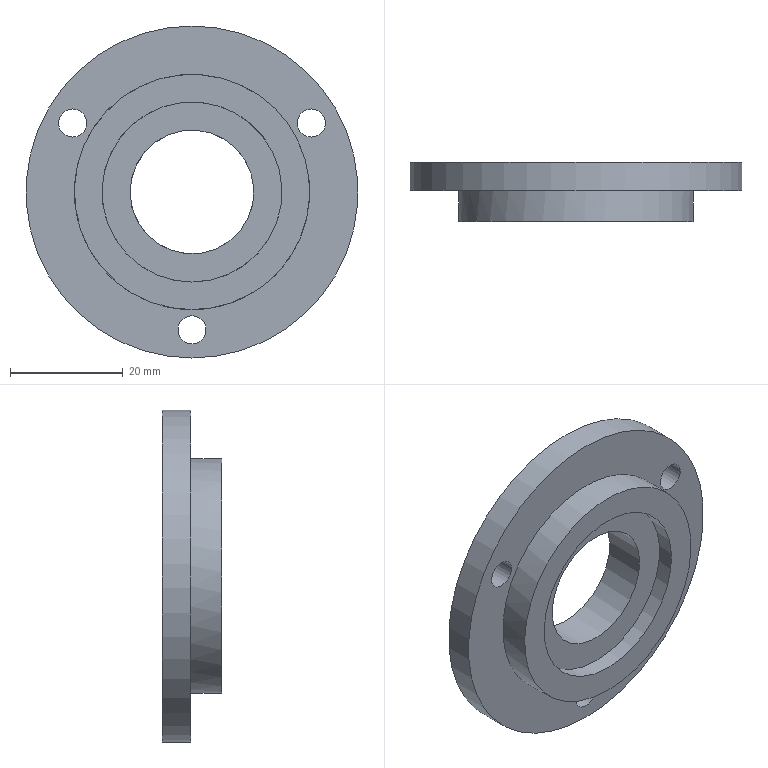Part | STEP file | YBQDJ-YB-13 | 1 solid | 11 faces | box 59 x 10.5 x 59 mm | volume 15659 mm3 | cylinder 7 | plane 4 | commonest cylinder face diameters 5 x3 22 x1 32 x1 41.8 x1 59 x1
STEP:
#1=CARTESIAN_POINT('',(0.,0.,0.));
#2=DIRECTION('',(0.,0.,1.));
#3=DIRECTION('',(1.,0.,0.));
#4=AXIS2_PLACEMENT_3D('',#1,#2,#3);
#5=CARTESIAN_POINT('',(-168.721,-90.,118.779));
#6=VERTEX_POINT('',#5);
#7=CARTESIAN_POINT('',(-183.5,-90.,104.));
#8=DIRECTION('',(0.,-1.,0.));
#9=DIRECTION('',(0.7071,0.,0.7071));
#10=AXIS2_PLACEMENT_3D('',#7,#8,#9);
#11=CIRCLE('',#10,20.9);
#12=CARTESIAN_POINT('',(-183.5,-95.,104.));
#13=DIRECTION('',(0.,1.,0.));
#14=DIRECTION('',(0.7071,0.,0.7071));
#15=AXIS2_PLACEMENT_3D('',#12,#13,#14);
#16=CYLINDRICAL_SURFACE('',#15,20.9);
#17=CARTESIAN_POINT('',(6.283,5.));
#18=DIRECTION('',(-1.,0.));
#19=VECTOR('',#18,1.);
#20=LINE('',#17,#19);
#21=(GEOMETRIC_REPRESENTATION_CONTEXT(2)PARAMETRIC_REPRESENTATION_CONTEXT()REPRESENTATION_CONTEXT('',''));
#22=DEFINITIONAL_REPRESENTATION('',(#20),#21);
#23=PCURVE('',#16,#22);
#24=CARTESIAN_POINT('',(-183.5,-90.,104.));
#25=DIRECTION('',(0.,-1.,0.));
#26=DIRECTION('',(-0.7071,0.,-0.7071));
#27=AXIS2_PLACEMENT_3D('',#24,#25,#26);
#28=PLANE('',#27);
#29=CARTESIAN_POINT('',(0.,0.));
#30=DIRECTION('',(-1.,0.));
#31=AXIS2_PLACEMENT_2D('',#29,#30);
#32=CIRCLE('',#31,20.9);
#33=(GEOMETRIC_REPRESENTATION_CONTEXT(2)PARAMETRIC_REPRESENTATION_CONTEXT()REPRESENTATION_CONTEXT('',''));
#34=DEFINITIONAL_REPRESENTATION('',(#32),#33);
#35=PCURVE('',#28,#34);
#36=SURFACE_CURVE('',#11,(#23,#35),.PCURVE_S1.);
#37=EDGE_CURVE('',#6,#6,#36,.T.);
#38=ORIENTED_EDGE('',*,*,#37,.T.);
#39=CARTESIAN_POINT('',(-168.721,-95.5,118.779));
#40=VERTEX_POINT('',#39);
#41=CARTESIAN_POINT('',(-168.721,-95.5,118.779));
#42=CARTESIAN_POINT('',(-168.721,-90.,118.779));
#43=B_SPLINE_CURVE_WITH_KNOTS('',1,(#41,#42),.UNSPECIFIED.,.F.,.F.,(2,2),(-0.5,5.),.PIECEWISE_BEZIER_KNOTS.);
#44=CARTESIAN_POINT('',(0.,0.));
#45=DIRECTION('',(0.,1.));
#46=VECTOR('',#45,1.);
#47=LINE('',#44,#46);
#48=(GEOMETRIC_REPRESENTATION_CONTEXT(2)PARAMETRIC_REPRESENTATION_CONTEXT()REPRESENTATION_CONTEXT('',''));
#49=DEFINITIONAL_REPRESENTATION('',(#47),#48);
#50=PCURVE('',#16,#49);
#51=CARTESIAN_POINT('',(6.283,0.));
#52=DIRECTION('',(0.,1.));
#53=VECTOR('',#52,1.);
#54=LINE('',#51,#53);
#55=(GEOMETRIC_REPRESENTATION_CONTEXT(2)PARAMETRIC_REPRESENTATION_CONTEXT()REPRESENTATION_CONTEXT('',''));
#56=DEFINITIONAL_REPRESENTATION('',(#54),#55);
#57=PCURVE('',#16,#56);
#58=SEAM_CURVE('',#43,(#50,#57),.PCURVE_S1.);
#59=EDGE_CURVE('',#40,#6,#58,.T.);
#60=ORIENTED_EDGE('',*,*,#59,.F.);
#61=CARTESIAN_POINT('',(-183.5,-95.5,83.1));
#62=VERTEX_POINT('',#61);
#63=CARTESIAN_POINT('',(-183.5,-95.5,104.));
#64=DIRECTION('',(0.,1.,0.));
#65=DIRECTION('',(0.,0.,-1.));
#66=AXIS2_PLACEMENT_3D('',#63,#64,#65);
#67=CIRCLE('',#66,20.9);
#68=CARTESIAN_POINT('',(-3.927,-0.5));
#69=DIRECTION('',(1.,0.));
#70=VECTOR('',#69,1.);
#71=LINE('',#68,#70);
#72=(GEOMETRIC_REPRESENTATION_CONTEXT(2)PARAMETRIC_REPRESENTATION_CONTEXT()REPRESENTATION_CONTEXT('',''));
#73=DEFINITIONAL_REPRESENTATION('',(#71),#72);
#74=PCURVE('',#16,#73);
#75=CARTESIAN_POINT('',(-183.5,-95.5,94.));
#76=DIRECTION('',(0.,1.,0.));
#77=DIRECTION('',(0.,0.,1.));
#78=AXIS2_PLACEMENT_3D('',#75,#76,#77);
#79=PLANE('',#78);
#80=CARTESIAN_POINT('',(10.,0.));
#81=DIRECTION('',(-1.,0.));
#82=AXIS2_PLACEMENT_2D('',#80,#81);
#83=CIRCLE('',#82,20.9);
#84=(GEOMETRIC_REPRESENTATION_CONTEXT(2)PARAMETRIC_REPRESENTATION_CONTEXT()REPRESENTATION_CONTEXT('',''));
#85=DEFINITIONAL_REPRESENTATION('',(#83),#84);
#86=PCURVE('',#79,#85);
#87=SURFACE_CURVE('',#67,(#74,#86),.PCURVE_S1.);
#88=EDGE_CURVE('',#40,#62,#87,.T.);
#89=ORIENTED_EDGE('',*,*,#88,.T.);
#90=CARTESIAN_POINT('',(-183.5,-95.5,104.));
#91=DIRECTION('',(0.,1.,0.));
#92=DIRECTION('',(0.,0.,-1.));
#93=AXIS2_PLACEMENT_3D('',#90,#91,#92);
#94=CIRCLE('',#93,20.9);
#95=CARTESIAN_POINT('',(2.356,-0.5));
#96=DIRECTION('',(1.,0.));
#97=VECTOR('',#96,1.);
#98=LINE('',#95,#97);
#99=(GEOMETRIC_REPRESENTATION_CONTEXT(2)PARAMETRIC_REPRESENTATION_CONTEXT()REPRESENTATION_CONTEXT('',''));
#100=DEFINITIONAL_REPRESENTATION('',(#98),#99);
#101=PCURVE('',#16,#100);
#102=CARTESIAN_POINT('',(10.,0.));
#103=DIRECTION('',(-1.,0.));
#104=AXIS2_PLACEMENT_2D('',#102,#103);
#105=CIRCLE('',#104,20.9);
#106=(GEOMETRIC_REPRESENTATION_CONTEXT(2)PARAMETRIC_REPRESENTATION_CONTEXT()REPRESENTATION_CONTEXT('',''));
#107=DEFINITIONAL_REPRESENTATION('',(#105),#106);
#108=PCURVE('',#79,#107);
#109=SURFACE_CURVE('',#94,(#101,#108),.PCURVE_S1.);
#110=EDGE_CURVE('',#62,#40,#109,.T.);
#111=ORIENTED_EDGE('',*,*,#110,.T.);
#112=ORIENTED_EDGE('',*,*,#59,.T.);
#113=EDGE_LOOP('',(#38,#60,#89,#111,#112));
#114=FACE_BOUND('',#113,.T.);
#115=ADVANCED_FACE('',(#114),#16,.T.);
#116=CARTESIAN_POINT('',(-183.5,-85.,133.5));
#117=VERTEX_POINT('',#116);
#118=CARTESIAN_POINT('',(-183.5,-85.,104.));
#119=DIRECTION('',(0.,1.,0.));
#120=DIRECTION('',(0.,0.,1.));
#121=AXIS2_PLACEMENT_3D('',#118,#119,#120);
#122=CIRCLE('',#121,29.5);
#123=CARTESIAN_POINT('',(-183.5,-85.,104.));
#124=DIRECTION('',(0.,-1.,0.));
#125=DIRECTION('',(-0.7071,0.,-0.7071));
#126=AXIS2_PLACEMENT_3D('',#123,#124,#125);
#127=CYLINDRICAL_SURFACE('',#126,29.5);
#128=CARTESIAN_POINT('',(10.21,0.));
#129=DIRECTION('',(-1.,0.));
#130=VECTOR('',#129,1.);
#131=LINE('',#128,#130);
#132=(GEOMETRIC_REPRESENTATION_CONTEXT(2)PARAMETRIC_REPRESENTATION_CONTEXT()REPRESENTATION_CONTEXT('',''));
#133=DEFINITIONAL_REPRESENTATION('',(#131),#132);
#134=PCURVE('',#127,#133);
#135=CARTESIAN_POINT('',(-183.5,-85.,104.));
#136=DIRECTION('',(0.,-1.,0.));
#137=DIRECTION('',(-0.7071,0.,-0.7071));
#138=AXIS2_PLACEMENT_3D('',#135,#136,#137);
#139=PLANE('',#138);
#140=CARTESIAN_POINT('',(-20.86,-20.86));
#141=CARTESIAN_POINT('',(-56.99,15.27));
#142=CARTESIAN_POINT('',(-7.635,28.495));
#143=CARTESIAN_POINT('',(41.719,41.719));
#144=CARTESIAN_POINT('',(28.495,-7.635));
#145=CARTESIAN_POINT('',(15.27,-56.99));
#146=CARTESIAN_POINT('',(-20.86,-20.86));
#147=(BOUNDED_CURVE()B_SPLINE_CURVE(2,(#140,#141,#142,#143,#144,#145,#146),.UNSPECIFIED.,.T.,.F.)B_SPLINE_CURVE_WITH_KNOTS((1,2,2,2,2,1),(-2.094,0.,2.094,4.189,6.283,8.378),.UNSPECIFIED.)CURVE()GEOMETRIC_REPRESENTATION_ITEM()RATIONAL_B_SPLINE_CURVE((1.,0.5,1.,0.5,1.,0.5,1.))REPRESENTATION_ITEM(''));
#148=(GEOMETRIC_REPRESENTATION_CONTEXT(2)PARAMETRIC_REPRESENTATION_CONTEXT()REPRESENTATION_CONTEXT('',''));
#149=DEFINITIONAL_REPRESENTATION('',(#147),#148);
#150=PCURVE('',#139,#149);
#151=SURFACE_CURVE('',#122,(#134,#150),.PCURVE_S1.);
#152=EDGE_CURVE('',#117,#117,#151,.T.);
#153=ORIENTED_EDGE('',*,*,#152,.F.);
#154=CARTESIAN_POINT('',(-183.5,-90.,133.5));
#155=VERTEX_POINT('',#154);
#156=CARTESIAN_POINT('',(-183.5,-85.,133.5));
#157=CARTESIAN_POINT('',(-183.5,-90.,133.5));
#158=B_SPLINE_CURVE_WITH_KNOTS('',1,(#156,#157),.UNSPECIFIED.,.F.,.F.,(2,2),(0.,5.),.PIECEWISE_BEZIER_KNOTS.);
#159=CARTESIAN_POINT('',(10.21,0.));
#160=DIRECTION('',(0.,1.));
#161=VECTOR('',#160,1.);
#162=LINE('',#159,#161);
#163=(GEOMETRIC_REPRESENTATION_CONTEXT(2)PARAMETRIC_REPRESENTATION_CONTEXT()REPRESENTATION_CONTEXT('',''));
#164=DEFINITIONAL_REPRESENTATION('',(#162),#163);
#165=PCURVE('',#127,#164);
#166=CARTESIAN_POINT('',(3.927,0.));
#167=DIRECTION('',(0.,1.));
#168=VECTOR('',#167,1.);
#169=LINE('',#166,#168);
#170=(GEOMETRIC_REPRESENTATION_CONTEXT(2)PARAMETRIC_REPRESENTATION_CONTEXT()REPRESENTATION_CONTEXT('',''));
#171=DEFINITIONAL_REPRESENTATION('',(#169),#170);
#172=PCURVE('',#127,#171);
#173=SEAM_CURVE('',#158,(#165,#172),.PCURVE_S1.);
#174=EDGE_CURVE('',#117,#155,#173,.T.);
#175=ORIENTED_EDGE('',*,*,#174,.T.);
#176=CARTESIAN_POINT('',(-183.5,-90.,104.));
#177=DIRECTION('',(0.,1.,0.));
#178=DIRECTION('',(0.,0.,1.));
#179=AXIS2_PLACEMENT_3D('',#176,#177,#178);
#180=CIRCLE('',#179,29.5);
#181=CARTESIAN_POINT('',(10.21,5.));
#182=DIRECTION('',(-1.,0.));
#183=VECTOR('',#182,1.);
#184=LINE('',#181,#183);
#185=(GEOMETRIC_REPRESENTATION_CONTEXT(2)PARAMETRIC_REPRESENTATION_CONTEXT()REPRESENTATION_CONTEXT('',''));
#186=DEFINITIONAL_REPRESENTATION('',(#184),#185);
#187=PCURVE('',#127,#186);
#188=CARTESIAN_POINT('',(-20.86,-20.86));
#189=CARTESIAN_POINT('',(-56.99,15.27));
#190=CARTESIAN_POINT('',(-7.635,28.495));
#191=CARTESIAN_POINT('',(41.719,41.719));
#192=CARTESIAN_POINT('',(28.495,-7.635));
#193=CARTESIAN_POINT('',(15.27,-56.99));
#194=CARTESIAN_POINT('',(-20.86,-20.86));
#195=(BOUNDED_CURVE()B_SPLINE_CURVE(2,(#188,#189,#190,#191,#192,#193,#194),.UNSPECIFIED.,.T.,.F.)B_SPLINE_CURVE_WITH_KNOTS((1,2,2,2,2,1),(-2.094,0.,2.094,4.189,6.283,8.378),.UNSPECIFIED.)CURVE()GEOMETRIC_REPRESENTATION_ITEM()RATIONAL_B_SPLINE_CURVE((1.,0.5,1.,0.5,1.,0.5,1.))REPRESENTATION_ITEM(''));
#196=(GEOMETRIC_REPRESENTATION_CONTEXT(2)PARAMETRIC_REPRESENTATION_CONTEXT()REPRESENTATION_CONTEXT('',''));
#197=DEFINITIONAL_REPRESENTATION('',(#195),#196);
#198=PCURVE('',#28,#197);
#199=SURFACE_CURVE('',#180,(#187,#198),.PCURVE_S1.);
#200=EDGE_CURVE('',#155,#155,#199,.T.);
#201=ORIENTED_EDGE('',*,*,#200,.T.);
#202=ORIENTED_EDGE('',*,*,#174,.F.);
#203=EDGE_LOOP('',(#153,#175,#201,#202));
#204=FACE_BOUND('',#203,.T.);
#205=ADVANCED_FACE('',(#204),#127,.T.);
#206=CARTESIAN_POINT('',(-204.718,-85.,118.75));
#207=VERTEX_POINT('',#206);
#208=CARTESIAN_POINT('',(-204.718,-85.,116.25));
#209=DIRECTION('',(0.,1.,0.));
#210=DIRECTION('',(0.,0.,1.));
#211=AXIS2_PLACEMENT_3D('',#208,#209,#210);
#212=CIRCLE('',#211,2.5);
#213=CARTESIAN_POINT('',(4.573,-25.433));
#214=CARTESIAN_POINT('',(1.511,-22.371));
#215=CARTESIAN_POINT('',(5.694,-21.25));
#216=CARTESIAN_POINT('',(9.877,-20.13));
#217=CARTESIAN_POINT('',(8.756,-24.312));
#218=CARTESIAN_POINT('',(7.635,-28.495));
#219=CARTESIAN_POINT('',(4.573,-25.433));
#220=(BOUNDED_CURVE()B_SPLINE_CURVE(2,(#213,#214,#215,#216,#217,#218,#219),.UNSPECIFIED.,.T.,.F.)B_SPLINE_CURVE_WITH_KNOTS((1,2,2,2,2,1),(-2.094,0.,2.094,4.189,6.283,8.378),.UNSPECIFIED.)CURVE()GEOMETRIC_REPRESENTATION_ITEM()RATIONAL_B_SPLINE_CURVE((1.,0.5,1.,0.5,1.,0.5,1.))REPRESENTATION_ITEM(''));
#221=(GEOMETRIC_REPRESENTATION_CONTEXT(2)PARAMETRIC_REPRESENTATION_CONTEXT()REPRESENTATION_CONTEXT('',''));
#222=DEFINITIONAL_REPRESENTATION('',(#220),#221);
#223=PCURVE('',#139,#222);
#224=CARTESIAN_POINT('',(-204.718,-97.2,116.25));
#225=DIRECTION('',(0.,1.,0.));
#226=DIRECTION('',(1.,0.,0.));
#227=AXIS2_PLACEMENT_3D('',#224,#225,#226);
#228=CYLINDRICAL_SURFACE('',#227,2.5);
#229=CARTESIAN_POINT('',(4.712,12.2));
#230=DIRECTION('',(1.,0.));
#231=VECTOR('',#230,1.);
#232=LINE('',#229,#231);
#233=(GEOMETRIC_REPRESENTATION_CONTEXT(2)PARAMETRIC_REPRESENTATION_CONTEXT()REPRESENTATION_CONTEXT('',''));
#234=DEFINITIONAL_REPRESENTATION('',(#232),#233);
#235=PCURVE('',#228,#234);
#236=SURFACE_CURVE('',#212,(#223,#235),.PCURVE_S1.);
#237=EDGE_CURVE('',#207,#207,#236,.T.);
#238=ORIENTED_EDGE('',*,*,#237,.F.);
#239=EDGE_LOOP('',(#238));
#240=FACE_BOUND('',#239,.T.);
#241=CARTESIAN_POINT('',(-183.5,-85.,82.));
#242=VERTEX_POINT('',#241);
#243=CARTESIAN_POINT('',(-183.5,-85.,79.5));
#244=DIRECTION('',(0.,1.,0.));
#245=DIRECTION('',(0.,0.,1.));
#246=AXIS2_PLACEMENT_3D('',#243,#244,#245);
#247=CIRCLE('',#246,2.5);
#248=CARTESIAN_POINT('',(15.556,15.556));
#249=CARTESIAN_POINT('',(12.494,18.618));
#250=CARTESIAN_POINT('',(16.677,19.739));
#251=CARTESIAN_POINT('',(20.86,20.86));
#252=CARTESIAN_POINT('',(19.739,16.677));
#253=CARTESIAN_POINT('',(18.618,12.494));
#254=CARTESIAN_POINT('',(15.556,15.556));
#255=(BOUNDED_CURVE()B_SPLINE_CURVE(2,(#248,#249,#250,#251,#252,#253,#254),.UNSPECIFIED.,.T.,.F.)B_SPLINE_CURVE_WITH_KNOTS((1,2,2,2,2,1),(-2.094,0.,2.094,4.189,6.283,8.378),.UNSPECIFIED.)CURVE()GEOMETRIC_REPRESENTATION_ITEM()RATIONAL_B_SPLINE_CURVE((1.,0.5,1.,0.5,1.,0.5,1.))REPRESENTATION_ITEM(''));
#256=(GEOMETRIC_REPRESENTATION_CONTEXT(2)PARAMETRIC_REPRESENTATION_CONTEXT()REPRESENTATION_CONTEXT('',''));
#257=DEFINITIONAL_REPRESENTATION('',(#255),#256);
#258=PCURVE('',#139,#257);
#259=CARTESIAN_POINT('',(-183.5,-97.2,79.5));
#260=DIRECTION('',(0.,1.,0.));
#261=DIRECTION('',(1.,0.,0.));
#262=AXIS2_PLACEMENT_3D('',#259,#260,#261);
#263=CYLINDRICAL_SURFACE('',#262,2.5);
#264=CARTESIAN_POINT('',(4.712,12.2));
#265=DIRECTION('',(1.,0.));
#266=VECTOR('',#265,1.);
#267=LINE('',#264,#266);
#268=(GEOMETRIC_REPRESENTATION_CONTEXT(2)PARAMETRIC_REPRESENTATION_CONTEXT()REPRESENTATION_CONTEXT('',''));
#269=DEFINITIONAL_REPRESENTATION('',(#267),#268);
#270=PCURVE('',#263,#269);
#271=SURFACE_CURVE('',#247,(#258,#270),.PCURVE_S1.);
#272=EDGE_CURVE('',#242,#242,#271,.T.);
#273=ORIENTED_EDGE('',*,*,#272,.F.);
#274=EDGE_LOOP('',(#273));
#275=FACE_BOUND('',#274,.T.);
#276=CARTESIAN_POINT('',(-162.282,-85.,118.75));
#277=VERTEX_POINT('',#276);
#278=CARTESIAN_POINT('',(-162.282,-85.,116.25));
#279=DIRECTION('',(0.,1.,0.));
#280=DIRECTION('',(0.,0.,1.));
#281=AXIS2_PLACEMENT_3D('',#278,#279,#280);
#282=CIRCLE('',#281,2.5);
#283=CARTESIAN_POINT('',(-25.433,4.573));
#284=CARTESIAN_POINT('',(-28.495,7.635));
#285=CARTESIAN_POINT('',(-24.312,8.756));
#286=CARTESIAN_POINT('',(-20.13,9.877));
#287=CARTESIAN_POINT('',(-21.25,5.694));
#288=CARTESIAN_POINT('',(-22.371,1.511));
#289=CARTESIAN_POINT('',(-25.433,4.573));
#290=(BOUNDED_CURVE()B_SPLINE_CURVE(2,(#283,#284,#285,#286,#287,#288,#289),.UNSPECIFIED.,.T.,.F.)B_SPLINE_CURVE_WITH_KNOTS((1,2,2,2,2,1),(-2.094,0.,2.094,4.189,6.283,8.378),.UNSPECIFIED.)CURVE()GEOMETRIC_REPRESENTATION_ITEM()RATIONAL_B_SPLINE_CURVE((1.,0.5,1.,0.5,1.,0.5,1.))REPRESENTATION_ITEM(''));
#291=(GEOMETRIC_REPRESENTATION_CONTEXT(2)PARAMETRIC_REPRESENTATION_CONTEXT()REPRESENTATION_CONTEXT('',''));
#292=DEFINITIONAL_REPRESENTATION('',(#290),#291);
#293=PCURVE('',#139,#292);
#294=CARTESIAN_POINT('',(-162.282,-97.2,116.25));
#295=DIRECTION('',(0.,1.,0.));
#296=DIRECTION('',(1.,0.,0.));
#297=AXIS2_PLACEMENT_3D('',#294,#295,#296);
#298=CYLINDRICAL_SURFACE('',#297,2.5);
#299=CARTESIAN_POINT('',(4.712,12.2));
#300=DIRECTION('',(1.,0.));
#301=VECTOR('',#300,1.);
#302=LINE('',#299,#301);
#303=(GEOMETRIC_REPRESENTATION_CONTEXT(2)PARAMETRIC_REPRESENTATION_CONTEXT()REPRESENTATION_CONTEXT('',''));
#304=DEFINITIONAL_REPRESENTATION('',(#302),#303);
#305=PCURVE('',#298,#304);
#306=SURFACE_CURVE('',#282,(#293,#305),.PCURVE_S1.);
#307=EDGE_CURVE('',#277,#277,#306,.T.);
#308=ORIENTED_EDGE('',*,*,#307,.F.);
#309=EDGE_LOOP('',(#308));
#310=FACE_BOUND('',#309,.T.);
#311=ORIENTED_EDGE('',*,*,#152,.T.);
#312=EDGE_LOOP('',(#311));
#313=FACE_BOUND('',#312,.T.);
#314=CARTESIAN_POINT('',(-175.722,-85.,111.778));
#315=VERTEX_POINT('',#314);
#316=CARTESIAN_POINT('',(-183.5,-85.,104.));
#317=DIRECTION('',(0.,-1.,0.));
#318=DIRECTION('',(0.7071,0.,0.7071));
#319=AXIS2_PLACEMENT_3D('',#316,#317,#318);
#320=CIRCLE('',#319,11.);
#321=CARTESIAN_POINT('',(0.,0.));
#322=DIRECTION('',(-1.,0.));
#323=AXIS2_PLACEMENT_2D('',#321,#322);
#324=CIRCLE('',#323,11.);
#325=(GEOMETRIC_REPRESENTATION_CONTEXT(2)PARAMETRIC_REPRESENTATION_CONTEXT()REPRESENTATION_CONTEXT('',''));
#326=DEFINITIONAL_REPRESENTATION('',(#324),#325);
#327=PCURVE('',#139,#326);
#328=CARTESIAN_POINT('',(-183.5,-95.,104.));
#329=DIRECTION('',(0.,1.,0.));
#330=DIRECTION('',(0.7071,0.,0.7071));
#331=AXIS2_PLACEMENT_3D('',#328,#329,#330);
#332=CYLINDRICAL_SURFACE('',#331,11.);
#333=CARTESIAN_POINT('',(6.283,10.));
#334=DIRECTION('',(-1.,0.));
#335=VECTOR('',#334,1.);
#336=LINE('',#333,#335);
#337=(GEOMETRIC_REPRESENTATION_CONTEXT(2)PARAMETRIC_REPRESENTATION_CONTEXT()REPRESENTATION_CONTEXT('',''));
#338=DEFINITIONAL_REPRESENTATION('',(#336),#337);
#339=PCURVE('',#332,#338);
#340=SURFACE_CURVE('',#320,(#327,#339),.PCURVE_S1.);
#341=EDGE_CURVE('',#315,#315,#340,.T.);
#342=ORIENTED_EDGE('',*,*,#341,.T.);
#343=EDGE_LOOP('',(#342));
#344=FACE_BOUND('',#343,.T.);
#345=ADVANCED_FACE('',(#240,#275,#310,#313,#344),#139,.F.);
#346=CARTESIAN_POINT('',(-204.718,-90.,118.75));
#347=VERTEX_POINT('',#346);
#348=CARTESIAN_POINT('',(-204.718,-90.,116.25));
#349=DIRECTION('',(0.,1.,0.));
#350=DIRECTION('',(0.,0.,1.));
#351=AXIS2_PLACEMENT_3D('',#348,#349,#350);
#352=CIRCLE('',#351,2.5);
#353=CARTESIAN_POINT('',(4.573,-25.433));
#354=CARTESIAN_POINT('',(1.511,-22.371));
#355=CARTESIAN_POINT('',(5.694,-21.25));
#356=CARTESIAN_POINT('',(9.877,-20.13));
#357=CARTESIAN_POINT('',(8.756,-24.312));
#358=CARTESIAN_POINT('',(7.635,-28.495));
#359=CARTESIAN_POINT('',(4.573,-25.433));
#360=(BOUNDED_CURVE()B_SPLINE_CURVE(2,(#353,#354,#355,#356,#357,#358,#359),.UNSPECIFIED.,.T.,.F.)B_SPLINE_CURVE_WITH_KNOTS((1,2,2,2,2,1),(-2.094,0.,2.094,4.189,6.283,8.378),.UNSPECIFIED.)CURVE()GEOMETRIC_REPRESENTATION_ITEM()RATIONAL_B_SPLINE_CURVE((1.,0.5,1.,0.5,1.,0.5,1.))REPRESENTATION_ITEM(''));
#361=(GEOMETRIC_REPRESENTATION_CONTEXT(2)PARAMETRIC_REPRESENTATION_CONTEXT()REPRESENTATION_CONTEXT('',''));
#362=DEFINITIONAL_REPRESENTATION('',(#360),#361);
#363=PCURVE('',#28,#362);
#364=CARTESIAN_POINT('',(4.712,7.2));
#365=DIRECTION('',(1.,0.));
#366=VECTOR('',#365,1.);
#367=LINE('',#364,#366);
#368=(GEOMETRIC_REPRESENTATION_CONTEXT(2)PARAMETRIC_REPRESENTATION_CONTEXT()REPRESENTATION_CONTEXT('',''));
#369=DEFINITIONAL_REPRESENTATION('',(#367),#368);
#370=PCURVE('',#228,#369);
#371=SURFACE_CURVE('',#352,(#363,#370),.PCURVE_S1.);
#372=EDGE_CURVE('',#347,#347,#371,.T.);
#373=ORIENTED_EDGE('',*,*,#372,.T.);
#374=EDGE_LOOP('',(#373));
#375=FACE_BOUND('',#374,.T.);
#376=CARTESIAN_POINT('',(-183.5,-90.,82.));
#377=VERTEX_POINT('',#376);
#378=CARTESIAN_POINT('',(-183.5,-90.,79.5));
#379=DIRECTION('',(0.,1.,0.));
#380=DIRECTION('',(0.,0.,1.));
#381=AXIS2_PLACEMENT_3D('',#378,#379,#380);
#382=CIRCLE('',#381,2.5);
#383=CARTESIAN_POINT('',(15.556,15.556));
#384=CARTESIAN_POINT('',(12.494,18.618));
#385=CARTESIAN_POINT('',(16.677,19.739));
#386=CARTESIAN_POINT('',(20.86,20.86));
#387=CARTESIAN_POINT('',(19.739,16.677));
#388=CARTESIAN_POINT('',(18.618,12.494));
#389=CARTESIAN_POINT('',(15.556,15.556));
#390=(BOUNDED_CURVE()B_SPLINE_CURVE(2,(#383,#384,#385,#386,#387,#388,#389),.UNSPECIFIED.,.T.,.F.)B_SPLINE_CURVE_WITH_KNOTS((1,2,2,2,2,1),(-2.094,0.,2.094,4.189,6.283,8.378),.UNSPECIFIED.)CURVE()GEOMETRIC_REPRESENTATION_ITEM()RATIONAL_B_SPLINE_CURVE((1.,0.5,1.,0.5,1.,0.5,1.))REPRESENTATION_ITEM(''));
#391=(GEOMETRIC_REPRESENTATION_CONTEXT(2)PARAMETRIC_REPRESENTATION_CONTEXT()REPRESENTATION_CONTEXT('',''));
#392=DEFINITIONAL_REPRESENTATION('',(#390),#391);
#393=PCURVE('',#28,#392);
#394=CARTESIAN_POINT('',(4.712,7.2));
#395=DIRECTION('',(1.,0.));
#396=VECTOR('',#395,1.);
#397=LINE('',#394,#396);
#398=(GEOMETRIC_REPRESENTATION_CONTEXT(2)PARAMETRIC_REPRESENTATION_CONTEXT()REPRESENTATION_CONTEXT('',''));
#399=DEFINITIONAL_REPRESENTATION('',(#397),#398);
#400=PCURVE('',#263,#399);
#401=SURFACE_CURVE('',#382,(#393,#400),.PCURVE_S1.);
#402=EDGE_CURVE('',#377,#377,#401,.T.);
#403=ORIENTED_EDGE('',*,*,#402,.T.);
#404=EDGE_LOOP('',(#403));
#405=FACE_BOUND('',#404,.T.);
#406=CARTESIAN_POINT('',(-162.282,-90.,118.75));
#407=VERTEX_POINT('',#406);
#408=CARTESIAN_POINT('',(-162.282,-90.,116.25));
#409=DIRECTION('',(0.,1.,0.));
#410=DIRECTION('',(0.,0.,1.));
#411=AXIS2_PLACEMENT_3D('',#408,#409,#410);
#412=CIRCLE('',#411,2.5);
#413=CARTESIAN_POINT('',(-25.433,4.573));
#414=CARTESIAN_POINT('',(-28.495,7.635));
#415=CARTESIAN_POINT('',(-24.312,8.756));
#416=CARTESIAN_POINT('',(-20.13,9.877));
#417=CARTESIAN_POINT('',(-21.25,5.694));
#418=CARTESIAN_POINT('',(-22.371,1.511));
#419=CARTESIAN_POINT('',(-25.433,4.573));
#420=(BOUNDED_CURVE()B_SPLINE_CURVE(2,(#413,#414,#415,#416,#417,#418,#419),.UNSPECIFIED.,.T.,.F.)B_SPLINE_CURVE_WITH_KNOTS((1,2,2,2,2,1),(-2.094,0.,2.094,4.189,6.283,8.378),.UNSPECIFIED.)CURVE()GEOMETRIC_REPRESENTATION_ITEM()RATIONAL_B_SPLINE_CURVE((1.,0.5,1.,0.5,1.,0.5,1.))REPRESENTATION_ITEM(''));
#421=(GEOMETRIC_REPRESENTATION_CONTEXT(2)PARAMETRIC_REPRESENTATION_CONTEXT()REPRESENTATION_CONTEXT('',''));
#422=DEFINITIONAL_REPRESENTATION('',(#420),#421);
#423=PCURVE('',#28,#422);
#424=CARTESIAN_POINT('',(4.712,7.2));
#425=DIRECTION('',(1.,0.));
#426=VECTOR('',#425,1.);
#427=LINE('',#424,#426);
#428=(GEOMETRIC_REPRESENTATION_CONTEXT(2)PARAMETRIC_REPRESENTATION_CONTEXT()REPRESENTATION_CONTEXT('',''));
#429=DEFINITIONAL_REPRESENTATION('',(#427),#428);
#430=PCURVE('',#298,#429);
#431=SURFACE_CURVE('',#412,(#423,#430),.PCURVE_S1.);
#432=EDGE_CURVE('',#407,#407,#431,.T.);
#433=ORIENTED_EDGE('',*,*,#432,.T.);
#434=EDGE_LOOP('',(#433));
#435=FACE_BOUND('',#434,.T.);
#436=ORIENTED_EDGE('',*,*,#200,.F.);
#437=EDGE_LOOP('',(#436));
#438=FACE_BOUND('',#437,.T.);
#439=ORIENTED_EDGE('',*,*,#37,.F.);
#440=EDGE_LOOP('',(#439));
#441=FACE_BOUND('',#440,.T.);
#442=ADVANCED_FACE('',(#375,#405,#435,#438,#441),#28,.T.);
#443=CARTESIAN_POINT('',(-183.5,-95.5,88.));
#444=VERTEX_POINT('',#443);
#445=CARTESIAN_POINT('',(-183.5,-95.5,104.));
#446=DIRECTION('',(0.,1.,0.));
#447=DIRECTION('',(0.,0.,-1.));
#448=AXIS2_PLACEMENT_3D('',#445,#446,#447);
#449=CIRCLE('',#448,16.);
#450=CARTESIAN_POINT('',(10.,0.));
#451=DIRECTION('',(-1.,0.));
#452=AXIS2_PLACEMENT_2D('',#450,#451);
#453=CIRCLE('',#452,16.);
#454=(GEOMETRIC_REPRESENTATION_CONTEXT(2)PARAMETRIC_REPRESENTATION_CONTEXT()REPRESENTATION_CONTEXT('',''));
#455=DEFINITIONAL_REPRESENTATION('',(#453),#454);
#456=PCURVE('',#79,#455);
#457=CARTESIAN_POINT('',(-183.5,-95.5,104.));
#458=DIRECTION('',(0.,1.,0.));
#459=DIRECTION('',(1.,0.,0.));
#460=AXIS2_PLACEMENT_3D('',#457,#458,#459);
#461=CYLINDRICAL_SURFACE('',#460,16.);
#462=CARTESIAN_POINT('',(1.571,0.));
#463=DIRECTION('',(1.,0.));
#464=VECTOR('',#463,1.);
#465=LINE('',#462,#464);
#466=(GEOMETRIC_REPRESENTATION_CONTEXT(2)PARAMETRIC_REPRESENTATION_CONTEXT()REPRESENTATION_CONTEXT('',''));
#467=DEFINITIONAL_REPRESENTATION('',(#465),#466);
#468=PCURVE('',#461,#467);
#469=SURFACE_CURVE('',#449,(#456,#468),.PCURVE_S1.);
#470=EDGE_CURVE('',#444,#444,#469,.T.);
#471=ORIENTED_EDGE('',*,*,#470,.T.);
#472=EDGE_LOOP('',(#471));
#473=FACE_BOUND('',#472,.T.);
#474=ORIENTED_EDGE('',*,*,#110,.F.);
#475=ORIENTED_EDGE('',*,*,#88,.F.);
#476=EDGE_LOOP('',(#474,#475));
#477=FACE_BOUND('',#476,.T.);
#478=ADVANCED_FACE('',(#473,#477),#79,.F.);
#479=CARTESIAN_POINT('',(-175.722,-92.5,111.778));
#480=VERTEX_POINT('',#479);
#481=CARTESIAN_POINT('',(-194.5,-92.5,104.));
#482=VERTEX_POINT('',#481);
#483=CARTESIAN_POINT('',(-183.5,-92.5,104.));
#484=DIRECTION('',(0.,-1.,0.));
#485=DIRECTION('',(-1.,0.,0.));
#486=AXIS2_PLACEMENT_3D('',#483,#484,#485);
#487=CIRCLE('',#486,11.);
#488=CARTESIAN_POINT('',(10.21,2.5));
#489=DIRECTION('',(-1.,0.));
#490=VECTOR('',#489,1.);
#491=LINE('',#488,#490);
#492=(GEOMETRIC_REPRESENTATION_CONTEXT(2)PARAMETRIC_REPRESENTATION_CONTEXT()REPRESENTATION_CONTEXT('',''));
#493=DEFINITIONAL_REPRESENTATION('',(#491),#492);
#494=PCURVE('',#332,#493);
#495=CARTESIAN_POINT('',(-183.5,-92.5,104.));
#496=DIRECTION('',(0.,1.,0.));
#497=DIRECTION('',(0.,0.,-1.));
#498=AXIS2_PLACEMENT_3D('',#495,#496,#497);
#499=PLANE('',#498);
#500=CARTESIAN_POINT('',(0.,11.));
#501=CARTESIAN_POINT('',(19.053,11.));
#502=CARTESIAN_POINT('',(9.526,-5.5));
#503=CARTESIAN_POINT('',(0.,-22.));
#504=CARTESIAN_POINT('',(-9.526,-5.5));
#505=CARTESIAN_POINT('',(-19.053,11.));
#506=CARTESIAN_POINT('',(0.,11.));
#507=(BOUNDED_CURVE()B_SPLINE_CURVE(2,(#500,#501,#502,#503,#504,#505,#506),.UNSPECIFIED.,.T.,.F.)B_SPLINE_CURVE_WITH_KNOTS((1,2,2,2,2,1),(-2.094,0.,2.094,4.189,6.283,8.378),.UNSPECIFIED.)CURVE()GEOMETRIC_REPRESENTATION_ITEM()RATIONAL_B_SPLINE_CURVE((1.,0.5,1.,0.5,1.,0.5,1.))REPRESENTATION_ITEM(''));
#508=(GEOMETRIC_REPRESENTATION_CONTEXT(2)PARAMETRIC_REPRESENTATION_CONTEXT()REPRESENTATION_CONTEXT('',''));
#509=DEFINITIONAL_REPRESENTATION('',(#507),#508);
#510=PCURVE('',#499,#509);
#511=SURFACE_CURVE('',#487,(#494,#510),.PCURVE_S1.);
#512=EDGE_CURVE('',#480,#482,#511,.T.);
#513=ORIENTED_EDGE('',*,*,#512,.F.);
#514=CARTESIAN_POINT('',(-175.722,-92.5,111.778));
#515=CARTESIAN_POINT('',(-175.722,-85.,111.778));
#516=B_SPLINE_CURVE_WITH_KNOTS('',1,(#514,#515),.UNSPECIFIED.,.F.,.F.,(2,2),(2.5,10.),.PIECEWISE_BEZIER_KNOTS.);
#517=CARTESIAN_POINT('',(6.283,0.));
#518=DIRECTION('',(0.,1.));
#519=VECTOR('',#518,1.);
#520=LINE('',#517,#519);
#521=(GEOMETRIC_REPRESENTATION_CONTEXT(2)PARAMETRIC_REPRESENTATION_CONTEXT()REPRESENTATION_CONTEXT('',''));
#522=DEFINITIONAL_REPRESENTATION('',(#520),#521);
#523=PCURVE('',#332,#522);
#524=CARTESIAN_POINT('',(0.,0.));
#525=DIRECTION('',(0.,1.));
#526=VECTOR('',#525,1.);
#527=LINE('',#524,#526);
#528=(GEOMETRIC_REPRESENTATION_CONTEXT(2)PARAMETRIC_REPRESENTATION_CONTEXT()REPRESENTATION_CONTEXT('',''));
#529=DEFINITIONAL_REPRESENTATION('',(#527),#528);
#530=PCURVE('',#332,#529);
#531=SEAM_CURVE('',#516,(#523,#530),.PCURVE_S1.);
#532=EDGE_CURVE('',#480,#315,#531,.T.);
#533=ORIENTED_EDGE('',*,*,#532,.T.);
#534=ORIENTED_EDGE('',*,*,#341,.T.);
#535=ORIENTED_EDGE('',*,*,#532,.F.);
#536=CARTESIAN_POINT('',(-183.5,-92.5,104.));
#537=DIRECTION('',(0.,-1.,0.));
#538=DIRECTION('',(-1.,0.,0.));
#539=AXIS2_PLACEMENT_3D('',#536,#537,#538);
#540=CIRCLE('',#539,11.);
#541=CARTESIAN_POINT('',(3.927,2.5));
#542=DIRECTION('',(-1.,0.));
#543=VECTOR('',#542,1.);
#544=LINE('',#541,#543);
#545=(GEOMETRIC_REPRESENTATION_CONTEXT(2)PARAMETRIC_REPRESENTATION_CONTEXT()REPRESENTATION_CONTEXT('',''));
#546=DEFINITIONAL_REPRESENTATION('',(#544),#545);
#547=PCURVE('',#332,#546);
#548=CARTESIAN_POINT('',(0.,11.));
#549=CARTESIAN_POINT('',(19.053,11.));
#550=CARTESIAN_POINT('',(9.526,-5.5));
#551=CARTESIAN_POINT('',(0.,-22.));
#552=CARTESIAN_POINT('',(-9.526,-5.5));
#553=CARTESIAN_POINT('',(-19.053,11.));
#554=CARTESIAN_POINT('',(0.,11.));
#555=(BOUNDED_CURVE()B_SPLINE_CURVE(2,(#548,#549,#550,#551,#552,#553,#554),.UNSPECIFIED.,.T.,.F.)B_SPLINE_CURVE_WITH_KNOTS((1,2,2,2,2,1),(-2.094,0.,2.094,4.189,6.283,8.378),.UNSPECIFIED.)CURVE()GEOMETRIC_REPRESENTATION_ITEM()RATIONAL_B_SPLINE_CURVE((1.,0.5,1.,0.5,1.,0.5,1.))REPRESENTATION_ITEM(''));
#556=(GEOMETRIC_REPRESENTATION_CONTEXT(2)PARAMETRIC_REPRESENTATION_CONTEXT()REPRESENTATION_CONTEXT('',''));
#557=DEFINITIONAL_REPRESENTATION('',(#555),#556);
#558=PCURVE('',#499,#557);
#559=SURFACE_CURVE('',#540,(#547,#558),.PCURVE_S1.);
#560=EDGE_CURVE('',#482,#480,#559,.T.);
#561=ORIENTED_EDGE('',*,*,#560,.F.);
#562=EDGE_LOOP('',(#513,#533,#534,#535,#561));
#563=FACE_BOUND('',#562,.F.);
#564=ADVANCED_FACE('',(#563),#332,.F.);
#565=CARTESIAN_POINT('',(-199.5,-92.5,104.));
#566=VERTEX_POINT('',#565);
#567=CARTESIAN_POINT('',(-183.5,-92.5,88.));
#568=VERTEX_POINT('',#567);
#569=CARTESIAN_POINT('',(-183.5,-92.5,104.));
#570=DIRECTION('',(0.,1.,0.));
#571=DIRECTION('',(-1.,0.,0.));
#572=AXIS2_PLACEMENT_3D('',#569,#570,#571);
#573=CIRCLE('',#572,16.);
#574=CARTESIAN_POINT('',(0.,0.));
#575=DIRECTION('',(0.,1.));
#576=AXIS2_PLACEMENT_2D('',#574,#575);
#577=CIRCLE('',#576,16.);
#578=(GEOMETRIC_REPRESENTATION_CONTEXT(2)PARAMETRIC_REPRESENTATION_CONTEXT()REPRESENTATION_CONTEXT('',''));
#579=DEFINITIONAL_REPRESENTATION('',(#577),#578);
#580=PCURVE('',#499,#579);
#581=CARTESIAN_POINT('',(3.142,3.));
#582=DIRECTION('',(1.,0.));
#583=VECTOR('',#582,1.);
#584=LINE('',#581,#583);
#585=(GEOMETRIC_REPRESENTATION_CONTEXT(2)PARAMETRIC_REPRESENTATION_CONTEXT()REPRESENTATION_CONTEXT('',''));
#586=DEFINITIONAL_REPRESENTATION('',(#584),#585);
#587=PCURVE('',#461,#586);
#588=SURFACE_CURVE('',#573,(#580,#587),.PCURVE_S1.);
#589=EDGE_CURVE('',#566,#568,#588,.T.);
#590=ORIENTED_EDGE('',*,*,#589,.F.);
#591=CARTESIAN_POINT('',(-183.5,-92.5,104.));
#592=DIRECTION('',(0.,1.,0.));
#593=DIRECTION('',(-1.,0.,0.));
#594=AXIS2_PLACEMENT_3D('',#591,#592,#593);
#595=CIRCLE('',#594,16.);
#596=CARTESIAN_POINT('',(0.,0.));
#597=DIRECTION('',(0.,1.));
#598=AXIS2_PLACEMENT_2D('',#596,#597);
#599=CIRCLE('',#598,16.);
#600=(GEOMETRIC_REPRESENTATION_CONTEXT(2)PARAMETRIC_REPRESENTATION_CONTEXT()REPRESENTATION_CONTEXT('',''));
#601=DEFINITIONAL_REPRESENTATION('',(#599),#600);
#602=PCURVE('',#499,#601);
#603=CARTESIAN_POINT('',(-3.142,3.));
#604=DIRECTION('',(1.,0.));
#605=VECTOR('',#604,1.);
#606=LINE('',#603,#605);
#607=(GEOMETRIC_REPRESENTATION_CONTEXT(2)PARAMETRIC_REPRESENTATION_CONTEXT()REPRESENTATION_CONTEXT('',''));
#608=DEFINITIONAL_REPRESENTATION('',(#606),#607);
#609=PCURVE('',#461,#608);
#610=SURFACE_CURVE('',#595,(#602,#609),.PCURVE_S1.);
#611=EDGE_CURVE('',#568,#566,#610,.T.);
#612=ORIENTED_EDGE('',*,*,#611,.F.);
#613=EDGE_LOOP('',(#590,#612));
#614=FACE_BOUND('',#613,.T.);
#615=ORIENTED_EDGE('',*,*,#560,.F.);
#616=ORIENTED_EDGE('',*,*,#512,.F.);
#617=EDGE_LOOP('',(#615,#616));
#618=FACE_BOUND('',#617,.T.);
#619=ADVANCED_FACE('',(#614,#618),#499,.F.);
#620=ORIENTED_EDGE('',*,*,#611,.F.);
#621=CARTESIAN_POINT('',(-183.5,-95.5,88.));
#622=CARTESIAN_POINT('',(-183.5,-92.5,88.));
#623=B_SPLINE_CURVE_WITH_KNOTS('',1,(#621,#622),.UNSPECIFIED.,.F.,.F.,(2,2),(0.,3.),.PIECEWISE_BEZIER_KNOTS.);
#624=CARTESIAN_POINT('',(1.571,0.));
#625=DIRECTION('',(0.,1.));
#626=VECTOR('',#625,1.);
#627=LINE('',#624,#626);
#628=(GEOMETRIC_REPRESENTATION_CONTEXT(2)PARAMETRIC_REPRESENTATION_CONTEXT()REPRESENTATION_CONTEXT('',''));
#629=DEFINITIONAL_REPRESENTATION('',(#627),#628);
#630=PCURVE('',#461,#629);
#631=CARTESIAN_POINT('',(7.854,0.));
#632=DIRECTION('',(0.,1.));
#633=VECTOR('',#632,1.);
#634=LINE('',#631,#633);
#635=(GEOMETRIC_REPRESENTATION_CONTEXT(2)PARAMETRIC_REPRESENTATION_CONTEXT()REPRESENTATION_CONTEXT('',''));
#636=DEFINITIONAL_REPRESENTATION('',(#634),#635);
#637=PCURVE('',#461,#636);
#638=SEAM_CURVE('',#623,(#630,#637),.PCURVE_S1.);
#639=EDGE_CURVE('',#444,#568,#638,.T.);
#640=ORIENTED_EDGE('',*,*,#639,.F.);
#641=ORIENTED_EDGE('',*,*,#470,.T.);
#642=ORIENTED_EDGE('',*,*,#639,.T.);
#643=ORIENTED_EDGE('',*,*,#589,.F.);
#644=EDGE_LOOP('',(#620,#640,#641,#642,#643));
#645=FACE_BOUND('',#644,.F.);
#646=ADVANCED_FACE('',(#645),#461,.F.);
#647=ORIENTED_EDGE('',*,*,#432,.T.);
#648=CARTESIAN_POINT('',(-162.282,-90.,118.75));
#649=CARTESIAN_POINT('',(-162.282,-85.,118.75));
#650=B_SPLINE_CURVE_WITH_KNOTS('',1,(#648,#649),.UNSPECIFIED.,.F.,.F.,(2,2),(7.2,12.2),.PIECEWISE_BEZIER_KNOTS.);
#651=CARTESIAN_POINT('',(10.996,0.));
#652=DIRECTION('',(0.,1.));
#653=VECTOR('',#652,1.);
#654=LINE('',#651,#653);
#655=(GEOMETRIC_REPRESENTATION_CONTEXT(2)PARAMETRIC_REPRESENTATION_CONTEXT()REPRESENTATION_CONTEXT('',''));
#656=DEFINITIONAL_REPRESENTATION('',(#654),#655);
#657=PCURVE('',#298,#656);
#658=CARTESIAN_POINT('',(4.712,0.));
#659=DIRECTION('',(0.,1.));
#660=VECTOR('',#659,1.);
#661=LINE('',#658,#660);
#662=(GEOMETRIC_REPRESENTATION_CONTEXT(2)PARAMETRIC_REPRESENTATION_CONTEXT()REPRESENTATION_CONTEXT('',''));
#663=DEFINITIONAL_REPRESENTATION('',(#661),#662);
#664=PCURVE('',#298,#663);
#665=SEAM_CURVE('',#650,(#657,#664),.PCURVE_S1.);
#666=EDGE_CURVE('',#407,#277,#665,.T.);
#667=ORIENTED_EDGE('',*,*,#666,.T.);
#668=ORIENTED_EDGE('',*,*,#307,.F.);
#669=ORIENTED_EDGE('',*,*,#666,.F.);
#670=EDGE_LOOP('',(#647,#667,#668,#669));
#671=FACE_BOUND('',#670,.F.);
#672=ADVANCED_FACE('',(#671),#298,.F.);
#673=ORIENTED_EDGE('',*,*,#402,.T.);
#674=CARTESIAN_POINT('',(-183.5,-90.,82.));
#675=CARTESIAN_POINT('',(-183.5,-85.,82.));
#676=B_SPLINE_CURVE_WITH_KNOTS('',1,(#674,#675),.UNSPECIFIED.,.F.,.F.,(2,2),(7.2,12.2),.PIECEWISE_BEZIER_KNOTS.);
#677=CARTESIAN_POINT('',(10.996,0.));
#678=DIRECTION('',(0.,1.));
#679=VECTOR('',#678,1.);
#680=LINE('',#677,#679);
#681=(GEOMETRIC_REPRESENTATION_CONTEXT(2)PARAMETRIC_REPRESENTATION_CONTEXT()REPRESENTATION_CONTEXT('',''));
#682=DEFINITIONAL_REPRESENTATION('',(#680),#681);
#683=PCURVE('',#263,#682);
#684=CARTESIAN_POINT('',(4.712,0.));
#685=DIRECTION('',(0.,1.));
#686=VECTOR('',#685,1.);
#687=LINE('',#684,#686);
#688=(GEOMETRIC_REPRESENTATION_CONTEXT(2)PARAMETRIC_REPRESENTATION_CONTEXT()REPRESENTATION_CONTEXT('',''));
#689=DEFINITIONAL_REPRESENTATION('',(#687),#688);
#690=PCURVE('',#263,#689);
#691=SEAM_CURVE('',#676,(#683,#690),.PCURVE_S1.);
#692=EDGE_CURVE('',#377,#242,#691,.T.);
#693=ORIENTED_EDGE('',*,*,#692,.T.);
#694=ORIENTED_EDGE('',*,*,#272,.F.);
#695=ORIENTED_EDGE('',*,*,#692,.F.);
#696=EDGE_LOOP('',(#673,#693,#694,#695));
#697=FACE_BOUND('',#696,.F.);
#698=ADVANCED_FACE('',(#697),#263,.F.);
#699=ORIENTED_EDGE('',*,*,#372,.T.);
#700=CARTESIAN_POINT('',(-204.718,-90.,118.75));
#701=CARTESIAN_POINT('',(-204.718,-85.,118.75));
#702=B_SPLINE_CURVE_WITH_KNOTS('',1,(#700,#701),.UNSPECIFIED.,.F.,.F.,(2,2),(7.2,12.2),.PIECEWISE_BEZIER_KNOTS.);
#703=CARTESIAN_POINT('',(10.996,0.));
#704=DIRECTION('',(0.,1.));
#705=VECTOR('',#704,1.);
#706=LINE('',#703,#705);
#707=(GEOMETRIC_REPRESENTATION_CONTEXT(2)PARAMETRIC_REPRESENTATION_CONTEXT()REPRESENTATION_CONTEXT('',''));
#708=DEFINITIONAL_REPRESENTATION('',(#706),#707);
#709=PCURVE('',#228,#708);
#710=CARTESIAN_POINT('',(4.712,0.));
#711=DIRECTION('',(0.,1.));
#712=VECTOR('',#711,1.);
#713=LINE('',#710,#712);
#714=(GEOMETRIC_REPRESENTATION_CONTEXT(2)PARAMETRIC_REPRESENTATION_CONTEXT()REPRESENTATION_CONTEXT('',''));
#715=DEFINITIONAL_REPRESENTATION('',(#713),#714);
#716=PCURVE('',#228,#715);
#717=SEAM_CURVE('',#702,(#709,#716),.PCURVE_S1.);
#718=EDGE_CURVE('',#347,#207,#717,.T.);
#719=ORIENTED_EDGE('',*,*,#718,.T.);
#720=ORIENTED_EDGE('',*,*,#237,.F.);
#721=ORIENTED_EDGE('',*,*,#718,.F.);
#722=EDGE_LOOP('',(#699,#719,#720,#721));
#723=FACE_BOUND('',#722,.F.);
#724=ADVANCED_FACE('',(#723),#228,.F.);
#725=CLOSED_SHELL('',(#115,#205,#345,#442,#478,#564,#619,#646,#672,#698,#724));
#726=MANIFOLD_SOLID_BREP('',#725);
#727=(LENGTH_UNIT()NAMED_UNIT(*)SI_UNIT(.MILLI.,.METRE.));
#728=UNCERTAINTY_MEASURE_WITH_UNIT(LENGTH_MEASURE(0.000005),#727,'','');
#729=(NAMED_UNIT(*)PLANE_ANGLE_UNIT()SI_UNIT($,.RADIAN.));
#730=(NAMED_UNIT(*)SI_UNIT($,.STERADIAN.)SOLID_ANGLE_UNIT());
#731=(GEOMETRIC_REPRESENTATION_CONTEXT(3)GLOBAL_UNCERTAINTY_ASSIGNED_CONTEXT((#728))GLOBAL_UNIT_ASSIGNED_CONTEXT((#727,#729,#730))REPRESENTATION_CONTEXT('',''));
#732=ADVANCED_BREP_SHAPE_REPRESENTATION('',(#4,#726),#731);